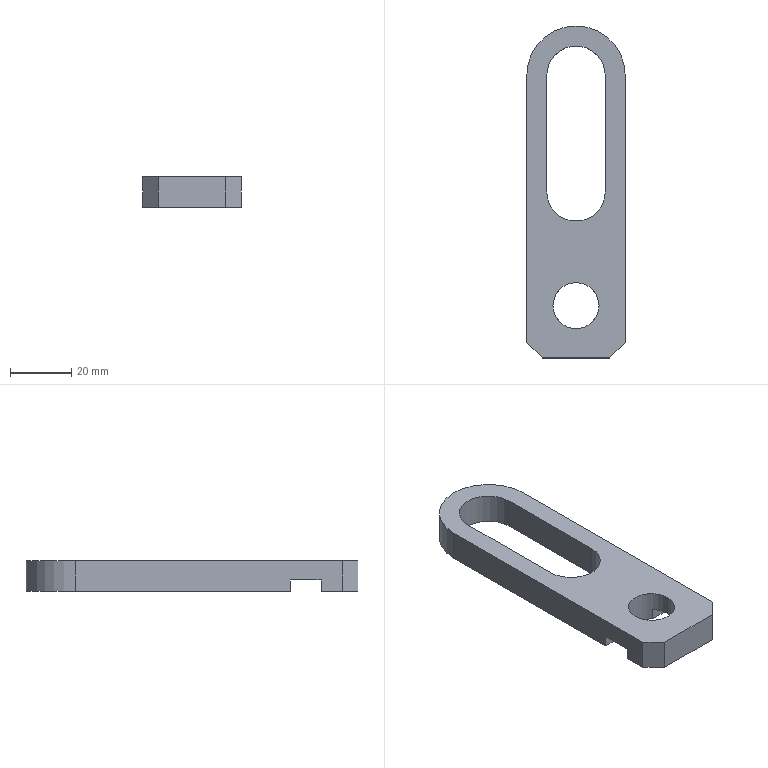Part | STEP file | 11-FG-E00511 | 1 solid | 22 faces | box 32 x 108 x 10 mm | volume 20715 mm3 | plane 16 | cylinder 6 | commonest cylinder face diameters 15 x2 19 x2 32 x2
STEP:
#1=CARTESIAN_POINT('',(-26.584,-50.307,10.));
#2=VERTEX_POINT('',#1);
#3=CARTESIAN_POINT('',(-41.584,-50.307,10.));
#4=VERTEX_POINT('',#3);
#5=CARTESIAN_POINT('',(-34.084,-50.307,10.));
#6=DIRECTION('',(0.,0.,-1.));
#7=DIRECTION('',(-1.,0.,0.));
#8=AXIS2_PLACEMENT_3D('',#5,#6,#7);
#9=CIRCLE('',#8,7.5);
#10=EDGE_CURVE('',#2,#4,#9,.T.);
#11=ORIENTED_EDGE('',*,*,#10,.F.);
#12=CARTESIAN_POINT('',(-26.584,-50.307,3.7));
#13=VERTEX_POINT('',#12);
#14=CARTESIAN_POINT('',(-26.584,-50.307,10.));
#15=DIRECTION('',(0.,0.,-1.));
#16=VECTOR('',#15,1000.);
#17=LINE('',#14,#16);
#18=EDGE_CURVE('',#2,#13,#17,.T.);
#19=ORIENTED_EDGE('',*,*,#18,.T.);
#20=CARTESIAN_POINT('',(-28.494,-55.307,3.7));
#21=VERTEX_POINT('',#20);
#22=CARTESIAN_POINT('',(-34.084,-50.307,3.7));
#23=DIRECTION('',(0.,0.,1.));
#24=DIRECTION('',(-1.,0.,0.));
#25=AXIS2_PLACEMENT_3D('',#22,#23,#24);
#26=CIRCLE('',#25,7.5);
#27=EDGE_CURVE('',#21,#13,#26,.T.);
#28=ORIENTED_EDGE('',*,*,#27,.F.);
#29=CARTESIAN_POINT('',(-28.494,-55.307,0.));
#30=VERTEX_POINT('',#29);
#31=CARTESIAN_POINT('',(-28.494,-55.307,10.));
#32=DIRECTION('',(0.,0.,-1.));
#33=VECTOR('',#32,1000.);
#34=LINE('',#31,#33);
#35=EDGE_CURVE('',#21,#30,#34,.T.);
#36=ORIENTED_EDGE('',*,*,#35,.T.);
#37=CARTESIAN_POINT('',(-39.675,-55.307,0.));
#38=VERTEX_POINT('',#37);
#39=CARTESIAN_POINT('',(-34.084,-50.307,0.));
#40=DIRECTION('',(0.,0.,-1.));
#41=DIRECTION('',(-1.,0.,0.));
#42=AXIS2_PLACEMENT_3D('',#39,#40,#41);
#43=CIRCLE('',#42,7.5);
#44=EDGE_CURVE('',#30,#38,#43,.T.);
#45=ORIENTED_EDGE('',*,*,#44,.T.);
#46=CARTESIAN_POINT('',(-39.675,-55.307,3.7));
#47=VERTEX_POINT('',#46);
#48=CARTESIAN_POINT('',(-39.675,-55.307,10.));
#49=DIRECTION('',(0.,0.,1.));
#50=VECTOR('',#49,1000.);
#51=LINE('',#48,#50);
#52=EDGE_CURVE('',#38,#47,#51,.T.);
#53=ORIENTED_EDGE('',*,*,#52,.T.);
#54=CARTESIAN_POINT('',(-41.584,-50.307,3.7));
#55=VERTEX_POINT('',#54);
#56=CARTESIAN_POINT('',(-34.084,-50.307,3.7));
#57=DIRECTION('',(0.,0.,1.));
#58=DIRECTION('',(-1.,0.,0.));
#59=AXIS2_PLACEMENT_3D('',#56,#57,#58);
#60=CIRCLE('',#59,7.5);
#61=EDGE_CURVE('',#55,#47,#60,.T.);
#62=ORIENTED_EDGE('',*,*,#61,.F.);
#63=CARTESIAN_POINT('',(-41.584,-50.307,10.));
#64=DIRECTION('',(0.,0.,-1.));
#65=VECTOR('',#64,1000.);
#66=LINE('',#63,#65);
#67=EDGE_CURVE('',#4,#55,#66,.T.);
#68=ORIENTED_EDGE('',*,*,#67,.F.);
#69=EDGE_LOOP('',(#11,#19,#28,#36,#45,#53,#62,#68));
#70=FACE_OUTER_BOUND('',#69,.T.);
#71=CARTESIAN_POINT('',(-34.084,-50.307,10.));
#72=DIRECTION('',(0.,0.,-1.));
#73=DIRECTION('',(-1.,0.,0.));
#74=AXIS2_PLACEMENT_3D('',#71,#72,#73);
#75=CYLINDRICAL_SURFACE('',#74,7.5);
#76=ADVANCED_FACE('',(#70),#75,.F.);
#77=CARTESIAN_POINT('',(-18.084,-62.307,0.));
#78=VERTEX_POINT('',#77);
#79=CARTESIAN_POINT('',(-18.084,-55.307,0.));
#80=VERTEX_POINT('',#79);
#81=CARTESIAN_POINT('',(-18.084,40.693,0.));
#82=DIRECTION('',(0.,1.,0.));
#83=VECTOR('',#82,1000.);
#84=LINE('',#81,#83);
#85=EDGE_CURVE('',#78,#80,#84,.T.);
#86=ORIENTED_EDGE('',*,*,#85,.F.);
#87=CARTESIAN_POINT('',(-23.084,-67.307,0.));
#88=VERTEX_POINT('',#87);
#89=CARTESIAN_POINT('',(-23.084,-67.307,0.));
#90=DIRECTION('',(-0.7071,-0.7071,0.));
#91=VECTOR('',#90,1000.);
#92=LINE('',#89,#91);
#93=EDGE_CURVE('',#78,#88,#92,.T.);
#94=ORIENTED_EDGE('',*,*,#93,.T.);
#95=CARTESIAN_POINT('',(-45.084,-67.307,0.));
#96=VERTEX_POINT('',#95);
#97=CARTESIAN_POINT('',(-50.084,-67.307,0.));
#98=DIRECTION('',(-1.,0.,0.));
#99=VECTOR('',#98,1000.);
#100=LINE('',#97,#99);
#101=EDGE_CURVE('',#88,#96,#100,.T.);
#102=ORIENTED_EDGE('',*,*,#101,.T.);
#103=CARTESIAN_POINT('',(-50.084,-62.307,0.));
#104=VERTEX_POINT('',#103);
#105=CARTESIAN_POINT('',(-50.084,-62.307,0.));
#106=DIRECTION('',(-0.7071,0.7071,0.));
#107=VECTOR('',#106,1000.);
#108=LINE('',#105,#107);
#109=EDGE_CURVE('',#96,#104,#108,.T.);
#110=ORIENTED_EDGE('',*,*,#109,.T.);
#111=CARTESIAN_POINT('',(-50.084,-55.307,0.));
#112=VERTEX_POINT('',#111);
#113=CARTESIAN_POINT('',(-50.084,40.693,0.));
#114=DIRECTION('',(0.,-1.,0.));
#115=VECTOR('',#114,1000.);
#116=LINE('',#113,#115);
#117=EDGE_CURVE('',#112,#104,#116,.T.);
#118=ORIENTED_EDGE('',*,*,#117,.F.);
#119=CARTESIAN_POINT('',(-12.897,-55.307,0.));
#120=DIRECTION('',(-1.,0.,0.));
#121=VECTOR('',#120,1000.);
#122=LINE('',#119,#121);
#123=EDGE_CURVE('',#38,#112,#122,.T.);
#124=ORIENTED_EDGE('',*,*,#123,.F.);
#125=ORIENTED_EDGE('',*,*,#44,.F.);
#126=CARTESIAN_POINT('',(-12.897,-55.307,0.));
#127=DIRECTION('',(-1.,0.,0.));
#128=VECTOR('',#127,1000.);
#129=LINE('',#126,#128);
#130=EDGE_CURVE('',#80,#30,#129,.T.);
#131=ORIENTED_EDGE('',*,*,#130,.F.);
#132=EDGE_LOOP('',(#86,#94,#102,#110,#118,#124,#125,#131));
#133=FACE_OUTER_BOUND('',#132,.T.);
#134=CARTESIAN_POINT('',(-50.084,-77.307,0.));
#135=DIRECTION('',(0.,0.,1.));
#136=DIRECTION('',(1.,0.,0.));
#137=AXIS2_PLACEMENT_3D('',#134,#135,#136);
#138=PLANE('',#137);
#139=ADVANCED_FACE('',(#133),#138,.F.);
#140=ORIENTED_EDGE('',*,*,#117,.T.);
#141=CARTESIAN_POINT('',(-50.084,-62.307,10.));
#142=VERTEX_POINT('',#141);
#143=CARTESIAN_POINT('',(-50.084,-62.307,10.));
#144=DIRECTION('',(0.,0.,1.));
#145=VECTOR('',#144,1000.);
#146=LINE('',#143,#145);
#147=EDGE_CURVE('',#104,#142,#146,.T.);
#148=ORIENTED_EDGE('',*,*,#147,.T.);
#149=CARTESIAN_POINT('',(-50.084,24.693,10.));
#150=VERTEX_POINT('',#149);
#151=CARTESIAN_POINT('',(-50.084,40.693,10.));
#152=DIRECTION('',(0.,-1.,0.));
#153=VECTOR('',#152,1000.);
#154=LINE('',#151,#153);
#155=EDGE_CURVE('',#150,#142,#154,.T.);
#156=ORIENTED_EDGE('',*,*,#155,.F.);
#157=CARTESIAN_POINT('',(-50.084,24.693,0.));
#158=VERTEX_POINT('',#157);
#159=CARTESIAN_POINT('',(-50.084,24.693,10.));
#160=DIRECTION('',(0.,0.,-1.));
#161=VECTOR('',#160,1000.);
#162=LINE('',#159,#161);
#163=EDGE_CURVE('',#150,#158,#162,.T.);
#164=ORIENTED_EDGE('',*,*,#163,.T.);
#165=CARTESIAN_POINT('',(-50.084,-45.307,0.));
#166=VERTEX_POINT('',#165);
#167=CARTESIAN_POINT('',(-50.084,40.693,0.));
#168=DIRECTION('',(0.,-1.,0.));
#169=VECTOR('',#168,1000.);
#170=LINE('',#167,#169);
#171=EDGE_CURVE('',#158,#166,#170,.T.);
#172=ORIENTED_EDGE('',*,*,#171,.T.);
#173=CARTESIAN_POINT('',(-50.084,-45.307,3.7));
#174=VERTEX_POINT('',#173);
#175=CARTESIAN_POINT('',(-50.084,-45.307,10.));
#176=DIRECTION('',(0.,0.,1.));
#177=VECTOR('',#176,1000.);
#178=LINE('',#175,#177);
#179=EDGE_CURVE('',#166,#174,#178,.T.);
#180=ORIENTED_EDGE('',*,*,#179,.T.);
#181=CARTESIAN_POINT('',(-50.084,-55.307,3.7));
#182=VERTEX_POINT('',#181);
#183=CARTESIAN_POINT('',(-50.084,40.693,3.7));
#184=DIRECTION('',(0.,1.,0.));
#185=VECTOR('',#184,1000.);
#186=LINE('',#183,#185);
#187=EDGE_CURVE('',#182,#174,#186,.T.);
#188=ORIENTED_EDGE('',*,*,#187,.F.);
#189=CARTESIAN_POINT('',(-50.084,-55.307,10.));
#190=DIRECTION('',(0.,0.,-1.));
#191=VECTOR('',#190,1000.);
#192=LINE('',#189,#191);
#193=EDGE_CURVE('',#182,#112,#192,.T.);
#194=ORIENTED_EDGE('',*,*,#193,.T.);
#195=EDGE_LOOP('',(#140,#148,#156,#164,#172,#180,#188,#194));
#196=FACE_OUTER_BOUND('',#195,.T.);
#197=CARTESIAN_POINT('',(-50.084,40.693,10.));
#198=DIRECTION('',(1.,0.,0.));
#199=DIRECTION('',(0.,1.,0.));
#200=AXIS2_PLACEMENT_3D('',#197,#198,#199);
#201=PLANE('',#200);
#202=ADVANCED_FACE('',(#196),#201,.F.);
#203=CARTESIAN_POINT('',(-18.084,-62.307,10.));
#204=VERTEX_POINT('',#203);
#205=CARTESIAN_POINT('',(-18.084,24.693,10.));
#206=VERTEX_POINT('',#205);
#207=CARTESIAN_POINT('',(-18.084,40.693,10.));
#208=DIRECTION('',(0.,1.,0.));
#209=VECTOR('',#208,1000.);
#210=LINE('',#207,#209);
#211=EDGE_CURVE('',#204,#206,#210,.T.);
#212=ORIENTED_EDGE('',*,*,#211,.F.);
#213=CARTESIAN_POINT('',(-18.084,-62.307,10.));
#214=DIRECTION('',(0.,0.,-1.));
#215=VECTOR('',#214,1000.);
#216=LINE('',#213,#215);
#217=EDGE_CURVE('',#204,#78,#216,.T.);
#218=ORIENTED_EDGE('',*,*,#217,.T.);
#219=ORIENTED_EDGE('',*,*,#85,.T.);
#220=CARTESIAN_POINT('',(-18.084,-55.307,3.7));
#221=VERTEX_POINT('',#220);
#222=CARTESIAN_POINT('',(-18.084,-55.307,10.));
#223=DIRECTION('',(0.,0.,1.));
#224=VECTOR('',#223,1000.);
#225=LINE('',#222,#224);
#226=EDGE_CURVE('',#80,#221,#225,.T.);
#227=ORIENTED_EDGE('',*,*,#226,.T.);
#228=CARTESIAN_POINT('',(-18.084,-45.307,3.7));
#229=VERTEX_POINT('',#228);
#230=CARTESIAN_POINT('',(-18.084,40.693,3.7));
#231=DIRECTION('',(0.,-1.,0.));
#232=VECTOR('',#231,1000.);
#233=LINE('',#230,#232);
#234=EDGE_CURVE('',#229,#221,#233,.T.);
#235=ORIENTED_EDGE('',*,*,#234,.F.);
#236=CARTESIAN_POINT('',(-18.084,-45.307,0.));
#237=VERTEX_POINT('',#236);
#238=CARTESIAN_POINT('',(-18.084,-45.307,10.));
#239=DIRECTION('',(0.,0.,-1.));
#240=VECTOR('',#239,1000.);
#241=LINE('',#238,#240);
#242=EDGE_CURVE('',#229,#237,#241,.T.);
#243=ORIENTED_EDGE('',*,*,#242,.T.);
#244=CARTESIAN_POINT('',(-18.084,24.693,0.));
#245=VERTEX_POINT('',#244);
#246=CARTESIAN_POINT('',(-18.084,40.693,0.));
#247=DIRECTION('',(0.,1.,0.));
#248=VECTOR('',#247,1000.);
#249=LINE('',#246,#248);
#250=EDGE_CURVE('',#237,#245,#249,.T.);
#251=ORIENTED_EDGE('',*,*,#250,.T.);
#252=CARTESIAN_POINT('',(-18.084,24.693,10.));
#253=DIRECTION('',(0.,0.,1.));
#254=VECTOR('',#253,1000.);
#255=LINE('',#252,#254);
#256=EDGE_CURVE('',#245,#206,#255,.T.);
#257=ORIENTED_EDGE('',*,*,#256,.T.);
#258=EDGE_LOOP('',(#212,#218,#219,#227,#235,#243,#251,#257));
#259=FACE_OUTER_BOUND('',#258,.T.);
#260=CARTESIAN_POINT('',(-18.084,40.693,10.));
#261=DIRECTION('',(-1.,0.,0.));
#262=DIRECTION('',(0.,-1.,0.));
#263=AXIS2_PLACEMENT_3D('',#260,#261,#262);
#264=PLANE('',#263);
#265=ADVANCED_FACE('',(#259),#264,.F.);
#266=CARTESIAN_POINT('',(-23.084,-67.307,10.));
#267=VERTEX_POINT('',#266);
#268=CARTESIAN_POINT('',(-45.084,-67.307,10.));
#269=VERTEX_POINT('',#268);
#270=CARTESIAN_POINT('',(-50.084,-67.307,10.));
#271=DIRECTION('',(-1.,0.,0.));
#272=VECTOR('',#271,1000.);
#273=LINE('',#270,#272);
#274=EDGE_CURVE('',#267,#269,#273,.T.);
#275=ORIENTED_EDGE('',*,*,#274,.F.);
#276=CARTESIAN_POINT('',(-41.584,-85.807,10.));
#277=DIRECTION('',(0.7071,0.7071,0.));
#278=VECTOR('',#277,1000.);
#279=LINE('',#276,#278);
#280=EDGE_CURVE('',#267,#204,#279,.T.);
#281=ORIENTED_EDGE('',*,*,#280,.T.);
#282=ORIENTED_EDGE('',*,*,#211,.T.);
#283=CARTESIAN_POINT('',(-34.084,40.693,10.));
#284=VERTEX_POINT('',#283);
#285=CARTESIAN_POINT('',(-34.084,24.693,10.));
#286=DIRECTION('',(0.,0.,1.));
#287=DIRECTION('',(1.,0.,0.));
#288=AXIS2_PLACEMENT_3D('',#285,#286,#287);
#289=CIRCLE('',#288,16.);
#290=EDGE_CURVE('',#206,#284,#289,.T.);
#291=ORIENTED_EDGE('',*,*,#290,.T.);
#292=CARTESIAN_POINT('',(-34.084,24.693,10.));
#293=DIRECTION('',(0.,0.,1.));
#294=DIRECTION('',(1.,0.,0.));
#295=AXIS2_PLACEMENT_3D('',#292,#293,#294);
#296=CIRCLE('',#295,16.);
#297=EDGE_CURVE('',#284,#150,#296,.T.);
#298=ORIENTED_EDGE('',*,*,#297,.T.);
#299=ORIENTED_EDGE('',*,*,#155,.T.);
#300=CARTESIAN_POINT('',(-42.584,-69.807,10.));
#301=DIRECTION('',(0.7071,-0.7071,0.));
#302=VECTOR('',#301,1000.);
#303=LINE('',#300,#302);
#304=EDGE_CURVE('',#142,#269,#303,.T.);
#305=ORIENTED_EDGE('',*,*,#304,.T.);
#306=EDGE_LOOP('',(#275,#281,#282,#291,#298,#299,#305));
#307=FACE_OUTER_BOUND('',#306,.T.);
#308=CARTESIAN_POINT('',(-34.084,-50.307,10.));
#309=DIRECTION('',(0.,0.,-1.));
#310=DIRECTION('',(-1.,0.,0.));
#311=AXIS2_PLACEMENT_3D('',#308,#309,#310);
#312=CIRCLE('',#311,7.5);
#313=EDGE_CURVE('',#4,#2,#312,.T.);
#314=ORIENTED_EDGE('',*,*,#313,.T.);
#315=ORIENTED_EDGE('',*,*,#10,.T.);
#316=EDGE_LOOP('',(#314,#315));
#317=FACE_BOUND('',#316,.T.);
#318=CARTESIAN_POINT('',(-24.584,24.693,10.));
#319=VERTEX_POINT('',#318);
#320=CARTESIAN_POINT('',(-43.584,24.693,10.));
#321=VERTEX_POINT('',#320);
#322=CARTESIAN_POINT('',(-34.084,24.693,10.));
#323=DIRECTION('',(0.,0.,1.));
#324=DIRECTION('',(1.,0.,0.));
#325=AXIS2_PLACEMENT_3D('',#322,#323,#324);
#326=CIRCLE('',#325,9.5);
#327=EDGE_CURVE('',#319,#321,#326,.T.);
#328=ORIENTED_EDGE('',*,*,#327,.F.);
#329=CARTESIAN_POINT('',(-24.584,-13.307,10.));
#330=VERTEX_POINT('',#329);
#331=CARTESIAN_POINT('',(-24.584,24.693,10.));
#332=DIRECTION('',(0.,1.,0.));
#333=VECTOR('',#332,1000.);
#334=LINE('',#331,#333);
#335=EDGE_CURVE('',#330,#319,#334,.T.);
#336=ORIENTED_EDGE('',*,*,#335,.F.);
#337=CARTESIAN_POINT('',(-43.584,-13.307,10.));
#338=VERTEX_POINT('',#337);
#339=CARTESIAN_POINT('',(-34.084,-13.307,10.));
#340=DIRECTION('',(0.,0.,1.));
#341=DIRECTION('',(1.,0.,0.));
#342=AXIS2_PLACEMENT_3D('',#339,#340,#341);
#343=CIRCLE('',#342,9.5);
#344=EDGE_CURVE('',#338,#330,#343,.T.);
#345=ORIENTED_EDGE('',*,*,#344,.F.);
#346=CARTESIAN_POINT('',(-43.584,24.693,10.));
#347=DIRECTION('',(0.,-1.,0.));
#348=VECTOR('',#347,1000.);
#349=LINE('',#346,#348);
#350=EDGE_CURVE('',#321,#338,#349,.T.);
#351=ORIENTED_EDGE('',*,*,#350,.F.);
#352=EDGE_LOOP('',(#328,#336,#345,#351));
#353=FACE_BOUND('',#352,.T.);
#354=CARTESIAN_POINT('',(-50.084,-77.307,10.));
#355=DIRECTION('',(0.,0.,1.));
#356=DIRECTION('',(1.,0.,0.));
#357=AXIS2_PLACEMENT_3D('',#354,#355,#356);
#358=PLANE('',#357);
#359=ADVANCED_FACE('',(#307,#317,#353),#358,.T.);
#360=ORIENTED_EDGE('',*,*,#250,.F.);
#361=CARTESIAN_POINT('',(-28.494,-45.307,0.));
#362=VERTEX_POINT('',#361);
#363=CARTESIAN_POINT('',(-12.897,-45.307,0.));
#364=DIRECTION('',(1.,0.,0.));
#365=VECTOR('',#364,1000.);
#366=LINE('',#363,#365);
#367=EDGE_CURVE('',#362,#237,#366,.T.);
#368=ORIENTED_EDGE('',*,*,#367,.F.);
#369=CARTESIAN_POINT('',(-39.675,-45.307,0.));
#370=VERTEX_POINT('',#369);
#371=CARTESIAN_POINT('',(-34.084,-50.307,0.));
#372=DIRECTION('',(0.,0.,-1.));
#373=DIRECTION('',(-1.,0.,0.));
#374=AXIS2_PLACEMENT_3D('',#371,#372,#373);
#375=CIRCLE('',#374,7.5);
#376=EDGE_CURVE('',#370,#362,#375,.T.);
#377=ORIENTED_EDGE('',*,*,#376,.F.);
#378=CARTESIAN_POINT('',(-12.897,-45.307,0.));
#379=DIRECTION('',(1.,0.,0.));
#380=VECTOR('',#379,1000.);
#381=LINE('',#378,#380);
#382=EDGE_CURVE('',#166,#370,#381,.T.);
#383=ORIENTED_EDGE('',*,*,#382,.F.);
#384=ORIENTED_EDGE('',*,*,#171,.F.);
#385=CARTESIAN_POINT('',(-34.084,40.693,0.));
#386=VERTEX_POINT('',#385);
#387=CARTESIAN_POINT('',(-34.084,24.693,0.));
#388=DIRECTION('',(0.,0.,-1.));
#389=DIRECTION('',(1.,0.,0.));
#390=AXIS2_PLACEMENT_3D('',#387,#388,#389);
#391=CIRCLE('',#390,16.);
#392=EDGE_CURVE('',#158,#386,#391,.T.);
#393=ORIENTED_EDGE('',*,*,#392,.T.);
#394=CARTESIAN_POINT('',(-34.084,24.693,0.));
#395=DIRECTION('',(0.,0.,-1.));
#396=DIRECTION('',(1.,0.,0.));
#397=AXIS2_PLACEMENT_3D('',#394,#395,#396);
#398=CIRCLE('',#397,16.);
#399=EDGE_CURVE('',#386,#245,#398,.T.);
#400=ORIENTED_EDGE('',*,*,#399,.T.);
#401=EDGE_LOOP('',(#360,#368,#377,#383,#384,#393,#400));
#402=FACE_OUTER_BOUND('',#401,.T.);
#403=CARTESIAN_POINT('',(-24.584,-13.307,0.));
#404=VERTEX_POINT('',#403);
#405=CARTESIAN_POINT('',(-24.584,24.693,0.));
#406=VERTEX_POINT('',#405);
#407=CARTESIAN_POINT('',(-24.584,24.693,0.));
#408=DIRECTION('',(0.,1.,0.));
#409=VECTOR('',#408,1000.);
#410=LINE('',#407,#409);
#411=EDGE_CURVE('',#404,#406,#410,.T.);
#412=ORIENTED_EDGE('',*,*,#411,.T.);
#413=CARTESIAN_POINT('',(-43.584,24.693,0.));
#414=VERTEX_POINT('',#413);
#415=CARTESIAN_POINT('',(-34.084,24.693,0.));
#416=DIRECTION('',(0.,0.,1.));
#417=DIRECTION('',(1.,0.,0.));
#418=AXIS2_PLACEMENT_3D('',#415,#416,#417);
#419=CIRCLE('',#418,9.5);
#420=EDGE_CURVE('',#406,#414,#419,.T.);
#421=ORIENTED_EDGE('',*,*,#420,.T.);
#422=CARTESIAN_POINT('',(-43.584,-13.307,0.));
#423=VERTEX_POINT('',#422);
#424=CARTESIAN_POINT('',(-43.584,24.693,0.));
#425=DIRECTION('',(0.,-1.,0.));
#426=VECTOR('',#425,1000.);
#427=LINE('',#424,#426);
#428=EDGE_CURVE('',#414,#423,#427,.T.);
#429=ORIENTED_EDGE('',*,*,#428,.T.);
#430=CARTESIAN_POINT('',(-34.084,-13.307,0.));
#431=DIRECTION('',(0.,0.,1.));
#432=DIRECTION('',(1.,0.,0.));
#433=AXIS2_PLACEMENT_3D('',#430,#431,#432);
#434=CIRCLE('',#433,9.5);
#435=EDGE_CURVE('',#423,#404,#434,.T.);
#436=ORIENTED_EDGE('',*,*,#435,.T.);
#437=EDGE_LOOP('',(#412,#421,#429,#436));
#438=FACE_BOUND('',#437,.T.);
#439=CARTESIAN_POINT('',(-50.084,-77.307,0.));
#440=DIRECTION('',(0.,0.,1.));
#441=DIRECTION('',(1.,0.,0.));
#442=AXIS2_PLACEMENT_3D('',#439,#440,#441);
#443=PLANE('',#442);
#444=ADVANCED_FACE('',(#402,#438),#443,.F.);
#445=ORIENTED_EDGE('',*,*,#327,.T.);
#446=CARTESIAN_POINT('',(-43.584,24.693,0.));
#447=DIRECTION('',(0.,0.,1.));
#448=VECTOR('',#447,1000.);
#449=LINE('',#446,#448);
#450=EDGE_CURVE('',#414,#321,#449,.T.);
#451=ORIENTED_EDGE('',*,*,#450,.F.);
#452=ORIENTED_EDGE('',*,*,#420,.F.);
#453=CARTESIAN_POINT('',(-24.584,24.693,0.));
#454=DIRECTION('',(0.,0.,1.));
#455=VECTOR('',#454,1000.);
#456=LINE('',#453,#455);
#457=EDGE_CURVE('',#406,#319,#456,.T.);
#458=ORIENTED_EDGE('',*,*,#457,.T.);
#459=EDGE_LOOP('',(#445,#451,#452,#458));
#460=FACE_OUTER_BOUND('',#459,.T.);
#461=CARTESIAN_POINT('',(-34.084,24.693,0.));
#462=DIRECTION('',(0.,0.,1.));
#463=DIRECTION('',(1.,0.,0.));
#464=AXIS2_PLACEMENT_3D('',#461,#462,#463);
#465=CYLINDRICAL_SURFACE('',#464,9.5);
#466=ADVANCED_FACE('',(#460),#465,.F.);
#467=ORIENTED_EDGE('',*,*,#335,.T.);
#468=ORIENTED_EDGE('',*,*,#457,.F.);
#469=ORIENTED_EDGE('',*,*,#411,.F.);
#470=CARTESIAN_POINT('',(-24.584,-13.307,0.));
#471=DIRECTION('',(0.,0.,1.));
#472=VECTOR('',#471,1000.);
#473=LINE('',#470,#472);
#474=EDGE_CURVE('',#404,#330,#473,.T.);
#475=ORIENTED_EDGE('',*,*,#474,.T.);
#476=EDGE_LOOP('',(#467,#468,#469,#475));
#477=FACE_OUTER_BOUND('',#476,.T.);
#478=CARTESIAN_POINT('',(-24.584,24.693,0.));
#479=DIRECTION('',(1.,0.,0.));
#480=DIRECTION('',(0.,0.,-1.));
#481=AXIS2_PLACEMENT_3D('',#478,#479,#480);
#482=PLANE('',#481);
#483=ADVANCED_FACE('',(#477),#482,.F.);
#484=ORIENTED_EDGE('',*,*,#344,.T.);
#485=ORIENTED_EDGE('',*,*,#474,.F.);
#486=ORIENTED_EDGE('',*,*,#435,.F.);
#487=CARTESIAN_POINT('',(-43.584,-13.307,0.));
#488=DIRECTION('',(0.,0.,1.));
#489=VECTOR('',#488,1000.);
#490=LINE('',#487,#489);
#491=EDGE_CURVE('',#423,#338,#490,.T.);
#492=ORIENTED_EDGE('',*,*,#491,.T.);
#493=EDGE_LOOP('',(#484,#485,#486,#492));
#494=FACE_OUTER_BOUND('',#493,.T.);
#495=CARTESIAN_POINT('',(-34.084,-13.307,0.));
#496=DIRECTION('',(0.,0.,1.));
#497=DIRECTION('',(1.,0.,0.));
#498=AXIS2_PLACEMENT_3D('',#495,#496,#497);
#499=CYLINDRICAL_SURFACE('',#498,9.5);
#500=ADVANCED_FACE('',(#494),#499,.F.);
#501=ORIENTED_EDGE('',*,*,#350,.T.);
#502=ORIENTED_EDGE('',*,*,#491,.F.);
#503=ORIENTED_EDGE('',*,*,#428,.F.);
#504=ORIENTED_EDGE('',*,*,#450,.T.);
#505=EDGE_LOOP('',(#501,#502,#503,#504));
#506=FACE_OUTER_BOUND('',#505,.T.);
#507=CARTESIAN_POINT('',(-43.584,24.693,0.));
#508=DIRECTION('',(-1.,0.,0.));
#509=DIRECTION('',(0.,-1.,0.));
#510=AXIS2_PLACEMENT_3D('',#507,#508,#509);
#511=PLANE('',#510);
#512=ADVANCED_FACE('',(#506),#511,.F.);
#513=CARTESIAN_POINT('',(-34.084,40.693,10.));
#514=DIRECTION('',(0.,0.,-1.));
#515=VECTOR('',#514,1000.);
#516=LINE('',#513,#515);
#517=EDGE_CURVE('',#284,#386,#516,.T.);
#518=ORIENTED_EDGE('',*,*,#517,.F.);
#519=ORIENTED_EDGE('',*,*,#290,.F.);
#520=ORIENTED_EDGE('',*,*,#256,.F.);
#521=ORIENTED_EDGE('',*,*,#399,.F.);
#522=EDGE_LOOP('',(#518,#519,#520,#521));
#523=FACE_OUTER_BOUND('',#522,.T.);
#524=CARTESIAN_POINT('',(-34.084,24.693,10.));
#525=DIRECTION('',(0.,0.,-1.));
#526=DIRECTION('',(-1.,0.,0.));
#527=AXIS2_PLACEMENT_3D('',#524,#525,#526);
#528=CYLINDRICAL_SURFACE('',#527,16.);
#529=ADVANCED_FACE('',(#523),#528,.T.);
#530=ORIENTED_EDGE('',*,*,#297,.F.);
#531=ORIENTED_EDGE('',*,*,#517,.T.);
#532=ORIENTED_EDGE('',*,*,#392,.F.);
#533=ORIENTED_EDGE('',*,*,#163,.F.);
#534=EDGE_LOOP('',(#530,#531,#532,#533));
#535=FACE_OUTER_BOUND('',#534,.T.);
#536=CARTESIAN_POINT('',(-34.084,24.693,10.));
#537=DIRECTION('',(0.,0.,-1.));
#538=DIRECTION('',(-1.,0.,0.));
#539=AXIS2_PLACEMENT_3D('',#536,#537,#538);
#540=CYLINDRICAL_SURFACE('',#539,16.);
#541=ADVANCED_FACE('',(#535),#540,.T.);
#542=ORIENTED_EDGE('',*,*,#18,.F.);
#543=ORIENTED_EDGE('',*,*,#313,.F.);
#544=ORIENTED_EDGE('',*,*,#67,.T.);
#545=CARTESIAN_POINT('',(-39.675,-45.307,3.7));
#546=VERTEX_POINT('',#545);
#547=CARTESIAN_POINT('',(-34.084,-50.307,3.7));
#548=DIRECTION('',(0.,0.,1.));
#549=DIRECTION('',(-1.,0.,0.));
#550=AXIS2_PLACEMENT_3D('',#547,#548,#549);
#551=CIRCLE('',#550,7.5);
#552=EDGE_CURVE('',#546,#55,#551,.T.);
#553=ORIENTED_EDGE('',*,*,#552,.F.);
#554=CARTESIAN_POINT('',(-39.675,-45.307,10.));
#555=DIRECTION('',(0.,0.,-1.));
#556=VECTOR('',#555,1000.);
#557=LINE('',#554,#556);
#558=EDGE_CURVE('',#546,#370,#557,.T.);
#559=ORIENTED_EDGE('',*,*,#558,.T.);
#560=ORIENTED_EDGE('',*,*,#376,.T.);
#561=CARTESIAN_POINT('',(-28.494,-45.307,3.7));
#562=VERTEX_POINT('',#561);
#563=CARTESIAN_POINT('',(-28.494,-45.307,10.));
#564=DIRECTION('',(0.,0.,1.));
#565=VECTOR('',#564,1000.);
#566=LINE('',#563,#565);
#567=EDGE_CURVE('',#362,#562,#566,.T.);
#568=ORIENTED_EDGE('',*,*,#567,.T.);
#569=CARTESIAN_POINT('',(-34.084,-50.307,3.7));
#570=DIRECTION('',(0.,0.,1.));
#571=DIRECTION('',(-1.,0.,0.));
#572=AXIS2_PLACEMENT_3D('',#569,#570,#571);
#573=CIRCLE('',#572,7.5);
#574=EDGE_CURVE('',#13,#562,#573,.T.);
#575=ORIENTED_EDGE('',*,*,#574,.F.);
#576=EDGE_LOOP('',(#542,#543,#544,#553,#559,#560,#568,#575));
#577=FACE_OUTER_BOUND('',#576,.T.);
#578=CARTESIAN_POINT('',(-34.084,-50.307,10.));
#579=DIRECTION('',(0.,0.,-1.));
#580=DIRECTION('',(-1.,0.,0.));
#581=AXIS2_PLACEMENT_3D('',#578,#579,#580);
#582=CYLINDRICAL_SURFACE('',#581,7.5);
#583=ADVANCED_FACE('',(#577),#582,.F.);
#584=ORIENTED_EDGE('',*,*,#101,.F.);
#585=CARTESIAN_POINT('',(-23.084,-67.307,-10.));
#586=DIRECTION('',(0.,0.,1.));
#587=VECTOR('',#586,1000.);
#588=LINE('',#585,#587);
#589=EDGE_CURVE('',#88,#267,#588,.T.);
#590=ORIENTED_EDGE('',*,*,#589,.T.);
#591=ORIENTED_EDGE('',*,*,#274,.T.);
#592=CARTESIAN_POINT('',(-45.084,-67.307,-10.));
#593=DIRECTION('',(0.,0.,-1.));
#594=VECTOR('',#593,1000.);
#595=LINE('',#592,#594);
#596=EDGE_CURVE('',#269,#96,#595,.T.);
#597=ORIENTED_EDGE('',*,*,#596,.T.);
#598=EDGE_LOOP('',(#584,#590,#591,#597));
#599=FACE_OUTER_BOUND('',#598,.T.);
#600=CARTESIAN_POINT('',(-50.084,-67.307,-10.));
#601=DIRECTION('',(0.,1.,0.));
#602=DIRECTION('',(0.,0.,1.));
#603=AXIS2_PLACEMENT_3D('',#600,#601,#602);
#604=PLANE('',#603);
#605=ADVANCED_FACE('',(#599),#604,.F.);
#606=ORIENTED_EDGE('',*,*,#187,.T.);
#607=CARTESIAN_POINT('',(-12.897,-45.307,3.7));
#608=DIRECTION('',(1.,0.,0.));
#609=VECTOR('',#608,1000.);
#610=LINE('',#607,#609);
#611=EDGE_CURVE('',#174,#546,#610,.T.);
#612=ORIENTED_EDGE('',*,*,#611,.T.);
#613=ORIENTED_EDGE('',*,*,#552,.T.);
#614=ORIENTED_EDGE('',*,*,#61,.T.);
#615=CARTESIAN_POINT('',(-12.897,-55.307,3.7));
#616=DIRECTION('',(-1.,0.,0.));
#617=VECTOR('',#616,1000.);
#618=LINE('',#615,#617);
#619=EDGE_CURVE('',#47,#182,#618,.T.);
#620=ORIENTED_EDGE('',*,*,#619,.T.);
#621=EDGE_LOOP('',(#606,#612,#613,#614,#620));
#622=FACE_OUTER_BOUND('',#621,.T.);
#623=CARTESIAN_POINT('',(0.,0.,3.7));
#624=DIRECTION('',(0.,0.,-1.));
#625=DIRECTION('',(-1.,0.,0.));
#626=AXIS2_PLACEMENT_3D('',#623,#624,#625);
#627=PLANE('',#626);
#628=ADVANCED_FACE('',(#622),#627,.T.);
#629=ORIENTED_EDGE('',*,*,#382,.T.);
#630=ORIENTED_EDGE('',*,*,#558,.F.);
#631=ORIENTED_EDGE('',*,*,#611,.F.);
#632=ORIENTED_EDGE('',*,*,#179,.F.);
#633=EDGE_LOOP('',(#629,#630,#631,#632));
#634=FACE_OUTER_BOUND('',#633,.T.);
#635=CARTESIAN_POINT('',(-12.897,-45.307,3.7));
#636=DIRECTION('',(0.,1.,0.));
#637=DIRECTION('',(0.,0.,1.));
#638=AXIS2_PLACEMENT_3D('',#635,#636,#637);
#639=PLANE('',#638);
#640=ADVANCED_FACE('',(#634),#639,.F.);
#641=ORIENTED_EDGE('',*,*,#619,.F.);
#642=ORIENTED_EDGE('',*,*,#52,.F.);
#643=ORIENTED_EDGE('',*,*,#123,.T.);
#644=ORIENTED_EDGE('',*,*,#193,.F.);
#645=EDGE_LOOP('',(#641,#642,#643,#644));
#646=FACE_OUTER_BOUND('',#645,.T.);
#647=CARTESIAN_POINT('',(-12.897,-55.307,3.7));
#648=DIRECTION('',(0.,-1.,0.));
#649=DIRECTION('',(0.,0.,-1.));
#650=AXIS2_PLACEMENT_3D('',#647,#648,#649);
#651=PLANE('',#650);
#652=ADVANCED_FACE('',(#646),#651,.F.);
#653=ORIENTED_EDGE('',*,*,#130,.T.);
#654=ORIENTED_EDGE('',*,*,#35,.F.);
#655=CARTESIAN_POINT('',(-12.897,-55.307,3.7));
#656=DIRECTION('',(-1.,0.,0.));
#657=VECTOR('',#656,1000.);
#658=LINE('',#655,#657);
#659=EDGE_CURVE('',#221,#21,#658,.T.);
#660=ORIENTED_EDGE('',*,*,#659,.F.);
#661=ORIENTED_EDGE('',*,*,#226,.F.);
#662=EDGE_LOOP('',(#653,#654,#660,#661));
#663=FACE_OUTER_BOUND('',#662,.T.);
#664=CARTESIAN_POINT('',(-12.897,-55.307,3.7));
#665=DIRECTION('',(0.,-1.,0.));
#666=DIRECTION('',(0.,0.,-1.));
#667=AXIS2_PLACEMENT_3D('',#664,#665,#666);
#668=PLANE('',#667);
#669=ADVANCED_FACE('',(#663),#668,.F.);
#670=CARTESIAN_POINT('',(-12.897,-45.307,3.7));
#671=DIRECTION('',(1.,0.,0.));
#672=VECTOR('',#671,1000.);
#673=LINE('',#670,#672);
#674=EDGE_CURVE('',#562,#229,#673,.T.);
#675=ORIENTED_EDGE('',*,*,#674,.F.);
#676=ORIENTED_EDGE('',*,*,#567,.F.);
#677=ORIENTED_EDGE('',*,*,#367,.T.);
#678=ORIENTED_EDGE('',*,*,#242,.F.);
#679=EDGE_LOOP('',(#675,#676,#677,#678));
#680=FACE_OUTER_BOUND('',#679,.T.);
#681=CARTESIAN_POINT('',(-12.897,-45.307,3.7));
#682=DIRECTION('',(0.,1.,0.));
#683=DIRECTION('',(0.,0.,1.));
#684=AXIS2_PLACEMENT_3D('',#681,#682,#683);
#685=PLANE('',#684);
#686=ADVANCED_FACE('',(#680),#685,.F.);
#687=ORIENTED_EDGE('',*,*,#234,.T.);
#688=ORIENTED_EDGE('',*,*,#659,.T.);
#689=ORIENTED_EDGE('',*,*,#27,.T.);
#690=ORIENTED_EDGE('',*,*,#574,.T.);
#691=ORIENTED_EDGE('',*,*,#674,.T.);
#692=EDGE_LOOP('',(#687,#688,#689,#690,#691));
#693=FACE_OUTER_BOUND('',#692,.T.);
#694=CARTESIAN_POINT('',(0.,0.,3.7));
#695=DIRECTION('',(0.,0.,-1.));
#696=DIRECTION('',(-1.,0.,0.));
#697=AXIS2_PLACEMENT_3D('',#694,#695,#696);
#698=PLANE('',#697);
#699=ADVANCED_FACE('',(#693),#698,.T.);
#700=ORIENTED_EDGE('',*,*,#93,.F.);
#701=ORIENTED_EDGE('',*,*,#217,.F.);
#702=ORIENTED_EDGE('',*,*,#280,.F.);
#703=ORIENTED_EDGE('',*,*,#589,.F.);
#704=EDGE_LOOP('',(#700,#701,#702,#703));
#705=FACE_OUTER_BOUND('',#704,.T.);
#706=CARTESIAN_POINT('',(-23.084,-67.307,-10.));
#707=DIRECTION('',(-0.7071,0.7071,0.));
#708=DIRECTION('',(0.,0.,1.));
#709=AXIS2_PLACEMENT_3D('',#706,#707,#708);
#710=PLANE('',#709);
#711=ADVANCED_FACE('',(#705),#710,.F.);
#712=ORIENTED_EDGE('',*,*,#109,.F.);
#713=ORIENTED_EDGE('',*,*,#596,.F.);
#714=ORIENTED_EDGE('',*,*,#304,.F.);
#715=ORIENTED_EDGE('',*,*,#147,.F.);
#716=EDGE_LOOP('',(#712,#713,#714,#715));
#717=FACE_OUTER_BOUND('',#716,.T.);
#718=CARTESIAN_POINT('',(-50.084,-62.307,10.));
#719=DIRECTION('',(0.7071,0.7071,0.));
#720=DIRECTION('',(0.,0.,1.));
#721=AXIS2_PLACEMENT_3D('',#718,#719,#720);
#722=PLANE('',#721);
#723=ADVANCED_FACE('',(#717),#722,.F.);
#724=CLOSED_SHELL('',(#76,#139,#202,#265,#359,#444,#466,#483,#500,#512,#529,#541,#583,#605,#628,#640,#652,#669,#686,#699,#711,#723));
#725=MANIFOLD_SOLID_BREP('',#724);
#726=CARTESIAN_POINT('',(0.,0.,0.));
#727=DIRECTION('',(0.,0.,1.));
#728=DIRECTION('',(1.,0.,0.));
#729=AXIS2_PLACEMENT_3D('',#726,#727,#728);
#730=(LENGTH_UNIT()NAMED_UNIT(*)SI_UNIT(.MILLI.,.METRE.));
#731=UNCERTAINTY_MEASURE_WITH_UNIT(LENGTH_MEASURE(0.00001),#730,'','');
#732=(NAMED_UNIT(*)PLANE_ANGLE_UNIT()SI_UNIT($,.RADIAN.));
#733=(NAMED_UNIT(*)SI_UNIT($,.STERADIAN.)SOLID_ANGLE_UNIT());
#734=(GEOMETRIC_REPRESENTATION_CONTEXT(3)GLOBAL_UNCERTAINTY_ASSIGNED_CONTEXT((#731))GLOBAL_UNIT_ASSIGNED_CONTEXT((#730,#732,#733))REPRESENTATION_CONTEXT('',''));
#735=ADVANCED_BREP_SHAPE_REPRESENTATION('',(#725,#729),#734);